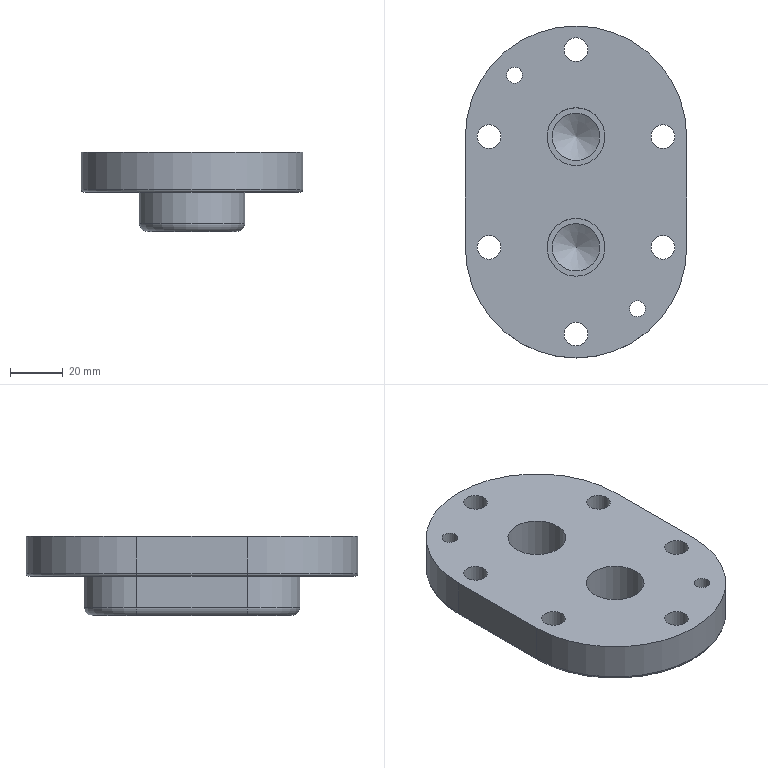Part | NX | features CBORE_HOLE 6, DATUM_CSYS 6, SKETCH 5, SIMPLE HOLE 4, EXTRUDE 3, HOLE PACKAGE 3, BLEND 2 | 1 solid | 45 faces | box 84 x 126 x 30 mm | volume 151500 mm3 | cylinder 24 | plane 15 | torus 4 | cone 2 | commonest cylinder face diameters 9 x6 15 x6 6 x4 2 x2 22 x2 40 x2
STEP:
#1=CARTESIAN_POINT('',(-42.,-21.,15.));
#2=VERTEX_POINT('',#1);
#3=CARTESIAN_POINT('',(-42.,-21.,1.));
#4=VERTEX_POINT('',#3);
#5=CARTESIAN_POINT('',(-42.,-21.,15.));
#6=DIRECTION('',(0.,0.,-1.));
#7=VECTOR('',#6,1000.);
#8=LINE('',#5,#7);
#9=EDGE_CURVE('',#2,#4,#8,.T.);
#10=ORIENTED_EDGE('',*,*,#9,.T.);
#11=CARTESIAN_POINT('',(42.,-21.,1.));
#12=VERTEX_POINT('',#11);
#13=CARTESIAN_POINT('',(0.,-21.,1.));
#14=DIRECTION('',(0.,0.,-1.));
#15=DIRECTION('',(-1.,0.,0.));
#16=AXIS2_PLACEMENT_3D('',#13,#14,#15);
#17=CIRCLE('',#16,42.);
#18=EDGE_CURVE('',#4,#12,#17,.F.);
#19=ORIENTED_EDGE('',*,*,#18,.T.);
#20=CARTESIAN_POINT('',(42.,-21.,15.));
#21=VERTEX_POINT('',#20);
#22=CARTESIAN_POINT('',(42.,-21.,15.));
#23=DIRECTION('',(0.,0.,-1.));
#24=VECTOR('',#23,1000.);
#25=LINE('',#22,#24);
#26=EDGE_CURVE('',#21,#12,#25,.T.);
#27=ORIENTED_EDGE('',*,*,#26,.F.);
#28=CARTESIAN_POINT('',(0.,-21.,15.));
#29=DIRECTION('',(0.,0.,-1.));
#30=DIRECTION('',(1.,0.,0.));
#31=AXIS2_PLACEMENT_3D('',#28,#29,#30);
#32=CIRCLE('',#31,42.);
#33=EDGE_CURVE('',#21,#2,#32,.T.);
#34=ORIENTED_EDGE('',*,*,#33,.T.);
#35=EDGE_LOOP('',(#10,#19,#27,#34));
#36=FACE_BOUND('',#35,.T.);
#37=CARTESIAN_POINT('',(0.,-21.,15.));
#38=DIRECTION('',(0.,0.,-1.));
#39=DIRECTION('',(-1.,0.,0.));
#40=AXIS2_PLACEMENT_3D('',#37,#38,#39);
#41=CYLINDRICAL_SURFACE('',#40,42.);
#42=ADVANCED_FACE('',(#36),#41,.T.);
#43=CARTESIAN_POINT('',(-42.,21.,15.));
#44=VERTEX_POINT('',#43);
#45=CARTESIAN_POINT('',(-42.,21.,1.));
#46=VERTEX_POINT('',#45);
#47=CARTESIAN_POINT('',(-42.,21.,15.));
#48=DIRECTION('',(0.,0.,-1.));
#49=VECTOR('',#48,1000.);
#50=LINE('',#47,#49);
#51=EDGE_CURVE('',#44,#46,#50,.T.);
#52=ORIENTED_EDGE('',*,*,#51,.T.);
#53=CARTESIAN_POINT('',(-42.,-21.,1.));
#54=DIRECTION('',(0.,1.,0.));
#55=VECTOR('',#54,1000.);
#56=LINE('',#53,#55);
#57=EDGE_CURVE('',#46,#4,#56,.F.);
#58=ORIENTED_EDGE('',*,*,#57,.T.);
#59=ORIENTED_EDGE('',*,*,#9,.F.);
#60=CARTESIAN_POINT('',(-42.,-21.,15.));
#61=DIRECTION('',(0.,1.,0.));
#62=VECTOR('',#61,1000.);
#63=LINE('',#60,#62);
#64=EDGE_CURVE('',#2,#44,#63,.T.);
#65=ORIENTED_EDGE('',*,*,#64,.T.);
#66=EDGE_LOOP('',(#52,#58,#59,#65));
#67=FACE_BOUND('',#66,.T.);
#68=CARTESIAN_POINT('',(-42.,-21.,15.));
#69=DIRECTION('',(-1.,0.,0.));
#70=DIRECTION('',(0.,-1.,0.));
#71=AXIS2_PLACEMENT_3D('',#68,#69,#70);
#72=PLANE('',#71);
#73=ADVANCED_FACE('',(#67),#72,.T.);
#74=CARTESIAN_POINT('',(42.,21.,15.));
#75=VERTEX_POINT('',#74);
#76=CARTESIAN_POINT('',(42.,21.,1.));
#77=VERTEX_POINT('',#76);
#78=CARTESIAN_POINT('',(42.,21.,15.));
#79=DIRECTION('',(0.,0.,-1.));
#80=VECTOR('',#79,1000.);
#81=LINE('',#78,#80);
#82=EDGE_CURVE('',#75,#77,#81,.T.);
#83=ORIENTED_EDGE('',*,*,#82,.T.);
#84=CARTESIAN_POINT('',(0.,21.,1.));
#85=DIRECTION('',(0.,0.,-1.));
#86=DIRECTION('',(-1.,0.,0.));
#87=AXIS2_PLACEMENT_3D('',#84,#85,#86);
#88=CIRCLE('',#87,42.);
#89=EDGE_CURVE('',#77,#46,#88,.F.);
#90=ORIENTED_EDGE('',*,*,#89,.T.);
#91=ORIENTED_EDGE('',*,*,#51,.F.);
#92=CARTESIAN_POINT('',(0.,21.,15.));
#93=DIRECTION('',(0.,0.,-1.));
#94=DIRECTION('',(1.,0.,0.));
#95=AXIS2_PLACEMENT_3D('',#92,#93,#94);
#96=CIRCLE('',#95,42.);
#97=EDGE_CURVE('',#44,#75,#96,.T.);
#98=ORIENTED_EDGE('',*,*,#97,.T.);
#99=EDGE_LOOP('',(#83,#90,#91,#98));
#100=FACE_BOUND('',#99,.T.);
#101=CARTESIAN_POINT('',(0.,21.,15.));
#102=DIRECTION('',(0.,0.,-1.));
#103=DIRECTION('',(-1.,0.,0.));
#104=AXIS2_PLACEMENT_3D('',#101,#102,#103);
#105=CYLINDRICAL_SURFACE('',#104,42.);
#106=ADVANCED_FACE('',(#100),#105,.T.);
#107=ORIENTED_EDGE('',*,*,#26,.T.);
#108=CARTESIAN_POINT('',(42.,21.,1.));
#109=DIRECTION('',(0.,-1.,0.));
#110=VECTOR('',#109,1000.);
#111=LINE('',#108,#110);
#112=EDGE_CURVE('',#12,#77,#111,.F.);
#113=ORIENTED_EDGE('',*,*,#112,.T.);
#114=ORIENTED_EDGE('',*,*,#82,.F.);
#115=CARTESIAN_POINT('',(42.,21.,15.));
#116=DIRECTION('',(0.,-1.,0.));
#117=VECTOR('',#116,1000.);
#118=LINE('',#115,#117);
#119=EDGE_CURVE('',#75,#21,#118,.T.);
#120=ORIENTED_EDGE('',*,*,#119,.T.);
#121=EDGE_LOOP('',(#107,#113,#114,#120));
#122=FACE_BOUND('',#121,.T.);
#123=CARTESIAN_POINT('',(42.,21.,15.));
#124=DIRECTION('',(1.,0.,0.));
#125=DIRECTION('',(0.,1.,0.));
#126=AXIS2_PLACEMENT_3D('',#123,#124,#125);
#127=PLANE('',#126);
#128=ADVANCED_FACE('',(#122),#127,.T.);
#129=CARTESIAN_POINT('',(20.335,-44.335,15.));
#130=VERTEX_POINT('',#129);
#131=CARTESIAN_POINT('',(23.335,-44.335,15.));
#132=DIRECTION('',(0.,0.,-1.));
#133=DIRECTION('',(-1.,0.,0.));
#134=AXIS2_PLACEMENT_3D('',#131,#132,#133);
#135=CIRCLE('',#134,3.);
#136=EDGE_CURVE('',#130,#130,#135,.T.);
#137=ORIENTED_EDGE('',*,*,#136,.T.);
#138=EDGE_LOOP('',(#137));
#139=FACE_BOUND('',#138,.T.);
#140=CARTESIAN_POINT('',(-26.335,44.335,15.));
#141=VERTEX_POINT('',#140);
#142=CARTESIAN_POINT('',(-23.335,44.335,15.));
#143=DIRECTION('',(0.,0.,-1.));
#144=DIRECTION('',(-1.,0.,0.));
#145=AXIS2_PLACEMENT_3D('',#142,#143,#144);
#146=CIRCLE('',#145,3.);
#147=EDGE_CURVE('',#141,#141,#146,.T.);
#148=ORIENTED_EDGE('',*,*,#147,.T.);
#149=EDGE_LOOP('',(#148));
#150=FACE_BOUND('',#149,.T.);
#151=CARTESIAN_POINT('',(28.5,21.,15.));
#152=VERTEX_POINT('',#151);
#153=CARTESIAN_POINT('',(33.,21.,15.));
#154=DIRECTION('',(0.,0.,-1.));
#155=DIRECTION('',(-1.,0.,0.));
#156=AXIS2_PLACEMENT_3D('',#153,#154,#155);
#157=CIRCLE('',#156,4.5);
#158=EDGE_CURVE('',#152,#152,#157,.T.);
#159=ORIENTED_EDGE('',*,*,#158,.T.);
#160=EDGE_LOOP('',(#159));
#161=FACE_BOUND('',#160,.T.);
#162=CARTESIAN_POINT('',(28.5,-21.,15.));
#163=VERTEX_POINT('',#162);
#164=CARTESIAN_POINT('',(33.,-21.,15.));
#165=DIRECTION('',(0.,0.,-1.));
#166=DIRECTION('',(-1.,0.,0.));
#167=AXIS2_PLACEMENT_3D('',#164,#165,#166);
#168=CIRCLE('',#167,4.5);
#169=EDGE_CURVE('',#163,#163,#168,.T.);
#170=ORIENTED_EDGE('',*,*,#169,.T.);
#171=EDGE_LOOP('',(#170));
#172=FACE_BOUND('',#171,.T.);
#173=CARTESIAN_POINT('',(-4.5,54.,15.));
#174=VERTEX_POINT('',#173);
#175=CARTESIAN_POINT('',(0.,54.,15.));
#176=DIRECTION('',(0.,0.,-1.));
#177=DIRECTION('',(-1.,0.,0.));
#178=AXIS2_PLACEMENT_3D('',#175,#176,#177);
#179=CIRCLE('',#178,4.5);
#180=EDGE_CURVE('',#174,#174,#179,.T.);
#181=ORIENTED_EDGE('',*,*,#180,.T.);
#182=EDGE_LOOP('',(#181));
#183=FACE_BOUND('',#182,.T.);
#184=CARTESIAN_POINT('',(-4.5,-54.,15.));
#185=VERTEX_POINT('',#184);
#186=CARTESIAN_POINT('',(0.,-54.,15.));
#187=DIRECTION('',(0.,0.,-1.));
#188=DIRECTION('',(-1.,0.,0.));
#189=AXIS2_PLACEMENT_3D('',#186,#187,#188);
#190=CIRCLE('',#189,4.5);
#191=EDGE_CURVE('',#185,#185,#190,.T.);
#192=ORIENTED_EDGE('',*,*,#191,.T.);
#193=EDGE_LOOP('',(#192));
#194=FACE_BOUND('',#193,.T.);
#195=CARTESIAN_POINT('',(-37.5,21.,15.));
#196=VERTEX_POINT('',#195);
#197=CARTESIAN_POINT('',(-33.,21.,15.));
#198=DIRECTION('',(0.,0.,-1.));
#199=DIRECTION('',(-1.,0.,0.));
#200=AXIS2_PLACEMENT_3D('',#197,#198,#199);
#201=CIRCLE('',#200,4.5);
#202=EDGE_CURVE('',#196,#196,#201,.T.);
#203=ORIENTED_EDGE('',*,*,#202,.T.);
#204=EDGE_LOOP('',(#203));
#205=FACE_BOUND('',#204,.T.);
#206=CARTESIAN_POINT('',(-37.5,-21.,15.));
#207=VERTEX_POINT('',#206);
#208=CARTESIAN_POINT('',(-33.,-21.,15.));
#209=DIRECTION('',(0.,0.,-1.));
#210=DIRECTION('',(-1.,0.,0.));
#211=AXIS2_PLACEMENT_3D('',#208,#209,#210);
#212=CIRCLE('',#211,4.5);
#213=EDGE_CURVE('',#207,#207,#212,.T.);
#214=ORIENTED_EDGE('',*,*,#213,.T.);
#215=EDGE_LOOP('',(#214));
#216=FACE_BOUND('',#215,.T.);
#217=CARTESIAN_POINT('',(0.,32.,15.));
#218=VERTEX_POINT('',#217);
#219=CARTESIAN_POINT('',(0.,21.,15.));
#220=DIRECTION('',(0.,0.,1.));
#221=DIRECTION('',(0.,1.,0.));
#222=AXIS2_PLACEMENT_3D('',#219,#220,#221);
#223=CIRCLE('',#222,11.);
#224=EDGE_CURVE('',#218,#218,#223,.T.);
#225=ORIENTED_EDGE('',*,*,#224,.F.);
#226=EDGE_LOOP('',(#225));
#227=FACE_BOUND('',#226,.T.);
#228=CARTESIAN_POINT('',(0.,-10.,15.));
#229=VERTEX_POINT('',#228);
#230=CARTESIAN_POINT('',(0.,-21.,15.));
#231=DIRECTION('',(0.,0.,1.));
#232=DIRECTION('',(0.,1.,0.));
#233=AXIS2_PLACEMENT_3D('',#230,#231,#232);
#234=CIRCLE('',#233,11.);
#235=EDGE_CURVE('',#229,#229,#234,.T.);
#236=ORIENTED_EDGE('',*,*,#235,.F.);
#237=EDGE_LOOP('',(#236));
#238=FACE_BOUND('',#237,.T.);
#239=ORIENTED_EDGE('',*,*,#33,.F.);
#240=ORIENTED_EDGE('',*,*,#119,.F.);
#241=ORIENTED_EDGE('',*,*,#97,.F.);
#242=ORIENTED_EDGE('',*,*,#64,.F.);
#243=EDGE_LOOP('',(#239,#240,#241,#242));
#244=FACE_BOUND('',#243,.T.);
#245=CARTESIAN_POINT('',(0.,-21.,15.));
#246=DIRECTION('',(0.,0.,-1.));
#247=DIRECTION('',(-1.,0.,0.));
#248=AXIS2_PLACEMENT_3D('',#245,#246,#247);
#249=PLANE('',#248);
#250=ADVANCED_FACE('',(#139,#150,#161,#172,#183,#194,#205,#216,#227,#238,#244),#249,.F.);
#251=CARTESIAN_POINT('',(26.335,-44.335,0.));
#252=VERTEX_POINT('',#251);
#253=CARTESIAN_POINT('',(23.335,-44.335,0.));
#254=DIRECTION('',(0.,0.,1.));
#255=DIRECTION('',(1.,0.,0.));
#256=AXIS2_PLACEMENT_3D('',#253,#254,#255);
#257=CIRCLE('',#256,3.);
#258=EDGE_CURVE('',#252,#252,#257,.T.);
#259=ORIENTED_EDGE('',*,*,#258,.T.);
#260=EDGE_LOOP('',(#259));
#261=FACE_BOUND('',#260,.T.);
#262=CARTESIAN_POINT('',(-20.335,44.335,0.));
#263=VERTEX_POINT('',#262);
#264=CARTESIAN_POINT('',(-23.335,44.335,0.));
#265=DIRECTION('',(0.,0.,1.));
#266=DIRECTION('',(1.,0.,0.));
#267=AXIS2_PLACEMENT_3D('',#264,#265,#266);
#268=CIRCLE('',#267,3.);
#269=EDGE_CURVE('',#263,#263,#268,.T.);
#270=ORIENTED_EDGE('',*,*,#269,.T.);
#271=EDGE_LOOP('',(#270));
#272=FACE_BOUND('',#271,.T.);
#273=CARTESIAN_POINT('',(-41.,21.,0.));
#274=VERTEX_POINT('',#273);
#275=CARTESIAN_POINT('',(41.,21.,0.));
#276=VERTEX_POINT('',#275);
#277=CARTESIAN_POINT('',(0.,21.,0.));
#278=DIRECTION('',(0.,0.,-1.));
#279=DIRECTION('',(-1.,0.,0.));
#280=AXIS2_PLACEMENT_3D('',#277,#278,#279);
#281=CIRCLE('',#280,41.);
#282=EDGE_CURVE('',#274,#276,#281,.T.);
#283=ORIENTED_EDGE('',*,*,#282,.T.);
#284=CARTESIAN_POINT('',(41.,-21.,0.));
#285=VERTEX_POINT('',#284);
#286=CARTESIAN_POINT('',(41.,-21.,0.));
#287=DIRECTION('',(0.,-1.,0.));
#288=VECTOR('',#287,1000.);
#289=LINE('',#286,#288);
#290=EDGE_CURVE('',#276,#285,#289,.T.);
#291=ORIENTED_EDGE('',*,*,#290,.T.);
#292=CARTESIAN_POINT('',(-41.,-21.,0.));
#293=VERTEX_POINT('',#292);
#294=CARTESIAN_POINT('',(0.,-21.,0.));
#295=DIRECTION('',(0.,0.,-1.));
#296=DIRECTION('',(-1.,0.,0.));
#297=AXIS2_PLACEMENT_3D('',#294,#295,#296);
#298=CIRCLE('',#297,41.);
#299=EDGE_CURVE('',#285,#293,#298,.T.);
#300=ORIENTED_EDGE('',*,*,#299,.T.);
#301=CARTESIAN_POINT('',(-41.,-21.,0.));
#302=DIRECTION('',(0.,1.,0.));
#303=VECTOR('',#302,1000.);
#304=LINE('',#301,#303);
#305=EDGE_CURVE('',#293,#274,#304,.T.);
#306=ORIENTED_EDGE('',*,*,#305,.T.);
#307=EDGE_LOOP('',(#283,#291,#300,#306));
#308=FACE_BOUND('',#307,.T.);
#309=CARTESIAN_POINT('',(40.5,21.,0.));
#310=VERTEX_POINT('',#309);
#311=CARTESIAN_POINT('',(33.,21.,0.));
#312=DIRECTION('',(0.,0.,1.));
#313=DIRECTION('',(1.,0.,0.));
#314=AXIS2_PLACEMENT_3D('',#311,#312,#313);
#315=CIRCLE('',#314,7.5);
#316=EDGE_CURVE('',#310,#310,#315,.T.);
#317=ORIENTED_EDGE('',*,*,#316,.T.);
#318=EDGE_LOOP('',(#317));
#319=FACE_BOUND('',#318,.T.);
#320=CARTESIAN_POINT('',(40.5,-21.,0.));
#321=VERTEX_POINT('',#320);
#322=CARTESIAN_POINT('',(33.,-21.,0.));
#323=DIRECTION('',(0.,0.,1.));
#324=DIRECTION('',(1.,0.,0.));
#325=AXIS2_PLACEMENT_3D('',#322,#323,#324);
#326=CIRCLE('',#325,7.5);
#327=EDGE_CURVE('',#321,#321,#326,.T.);
#328=ORIENTED_EDGE('',*,*,#327,.T.);
#329=EDGE_LOOP('',(#328));
#330=FACE_BOUND('',#329,.T.);
#331=CARTESIAN_POINT('',(7.5,54.,0.));
#332=VERTEX_POINT('',#331);
#333=CARTESIAN_POINT('',(0.,54.,0.));
#334=DIRECTION('',(0.,0.,1.));
#335=DIRECTION('',(1.,0.,0.));
#336=AXIS2_PLACEMENT_3D('',#333,#334,#335);
#337=CIRCLE('',#336,7.5);
#338=EDGE_CURVE('',#332,#332,#337,.T.);
#339=ORIENTED_EDGE('',*,*,#338,.T.);
#340=EDGE_LOOP('',(#339));
#341=FACE_BOUND('',#340,.T.);
#342=CARTESIAN_POINT('',(7.5,-54.,0.));
#343=VERTEX_POINT('',#342);
#344=CARTESIAN_POINT('',(0.,-54.,0.));
#345=DIRECTION('',(0.,0.,1.));
#346=DIRECTION('',(1.,0.,0.));
#347=AXIS2_PLACEMENT_3D('',#344,#345,#346);
#348=CIRCLE('',#347,7.5);
#349=EDGE_CURVE('',#343,#343,#348,.T.);
#350=ORIENTED_EDGE('',*,*,#349,.T.);
#351=EDGE_LOOP('',(#350));
#352=FACE_BOUND('',#351,.T.);
#353=CARTESIAN_POINT('',(-25.5,21.,0.));
#354=VERTEX_POINT('',#353);
#355=CARTESIAN_POINT('',(-33.,21.,0.));
#356=DIRECTION('',(0.,0.,1.));
#357=DIRECTION('',(1.,0.,0.));
#358=AXIS2_PLACEMENT_3D('',#355,#356,#357);
#359=CIRCLE('',#358,7.5);
#360=EDGE_CURVE('',#354,#354,#359,.T.);
#361=ORIENTED_EDGE('',*,*,#360,.T.);
#362=EDGE_LOOP('',(#361));
#363=FACE_BOUND('',#362,.T.);
#364=CARTESIAN_POINT('',(-25.5,-21.,0.));
#365=VERTEX_POINT('',#364);
#366=CARTESIAN_POINT('',(-33.,-21.,0.));
#367=DIRECTION('',(0.,0.,1.));
#368=DIRECTION('',(1.,0.,0.));
#369=AXIS2_PLACEMENT_3D('',#366,#367,#368);
#370=CIRCLE('',#369,7.5);
#371=EDGE_CURVE('',#365,#365,#370,.T.);
#372=ORIENTED_EDGE('',*,*,#371,.T.);
#373=EDGE_LOOP('',(#372));
#374=FACE_BOUND('',#373,.T.);
#375=CARTESIAN_POINT('',(-20.,-21.,0.));
#376=VERTEX_POINT('',#375);
#377=CARTESIAN_POINT('',(-20.,21.,0.));
#378=VERTEX_POINT('',#377);
#379=CARTESIAN_POINT('',(-20.,-21.,0.));
#380=DIRECTION('',(0.,1.,0.));
#381=VECTOR('',#380,1000.);
#382=LINE('',#379,#381);
#383=EDGE_CURVE('',#376,#378,#382,.T.);
#384=ORIENTED_EDGE('',*,*,#383,.F.);
#385=CARTESIAN_POINT('',(20.,-21.,0.));
#386=VERTEX_POINT('',#385);
#387=CARTESIAN_POINT('',(0.,-21.,0.));
#388=DIRECTION('',(0.,0.,-1.));
#389=DIRECTION('',(1.,0.,0.));
#390=AXIS2_PLACEMENT_3D('',#387,#388,#389);
#391=CIRCLE('',#390,20.);
#392=EDGE_CURVE('',#386,#376,#391,.T.);
#393=ORIENTED_EDGE('',*,*,#392,.F.);
#394=CARTESIAN_POINT('',(20.,21.,0.));
#395=VERTEX_POINT('',#394);
#396=CARTESIAN_POINT('',(20.,21.,0.));
#397=DIRECTION('',(0.,-1.,0.));
#398=VECTOR('',#397,1000.);
#399=LINE('',#396,#398);
#400=EDGE_CURVE('',#395,#386,#399,.T.);
#401=ORIENTED_EDGE('',*,*,#400,.F.);
#402=CARTESIAN_POINT('',(0.,21.,0.));
#403=DIRECTION('',(0.,0.,-1.));
#404=DIRECTION('',(1.,0.,0.));
#405=AXIS2_PLACEMENT_3D('',#402,#403,#404);
#406=CIRCLE('',#405,20.);
#407=EDGE_CURVE('',#378,#395,#406,.T.);
#408=ORIENTED_EDGE('',*,*,#407,.F.);
#409=EDGE_LOOP('',(#384,#393,#401,#408));
#410=FACE_BOUND('',#409,.T.);
#411=CARTESIAN_POINT('',(0.,-21.,0.));
#412=DIRECTION('',(0.,0.,-1.));
#413=DIRECTION('',(-1.,0.,0.));
#414=AXIS2_PLACEMENT_3D('',#411,#412,#413);
#415=PLANE('',#414);
#416=ADVANCED_FACE('',(#261,#272,#308,#319,#330,#341,#352,#363,#374,#410),#415,.T.);
#417=CARTESIAN_POINT('',(-20.,21.,-12.));
#418=VERTEX_POINT('',#417);
#419=CARTESIAN_POINT('',(-20.,21.,-15.));
#420=DIRECTION('',(0.,0.,1.));
#421=VECTOR('',#420,1000.);
#422=LINE('',#419,#421);
#423=EDGE_CURVE('',#418,#378,#422,.T.);
#424=ORIENTED_EDGE('',*,*,#423,.F.);
#425=CARTESIAN_POINT('',(-20.,-21.,-12.));
#426=VERTEX_POINT('',#425);
#427=CARTESIAN_POINT('',(-20.,-21.,-12.));
#428=DIRECTION('',(0.,1.,0.));
#429=VECTOR('',#428,1000.);
#430=LINE('',#427,#429);
#431=EDGE_CURVE('',#418,#426,#430,.F.);
#432=ORIENTED_EDGE('',*,*,#431,.T.);
#433=CARTESIAN_POINT('',(-20.,-21.,-15.));
#434=DIRECTION('',(0.,0.,1.));
#435=VECTOR('',#434,1000.);
#436=LINE('',#433,#435);
#437=EDGE_CURVE('',#426,#376,#436,.T.);
#438=ORIENTED_EDGE('',*,*,#437,.T.);
#439=ORIENTED_EDGE('',*,*,#383,.T.);
#440=EDGE_LOOP('',(#424,#432,#438,#439));
#441=FACE_BOUND('',#440,.T.);
#442=CARTESIAN_POINT('',(-20.,-21.,-15.));
#443=DIRECTION('',(1.,0.,0.));
#444=DIRECTION('',(0.,1.,0.));
#445=AXIS2_PLACEMENT_3D('',#442,#443,#444);
#446=PLANE('',#445);
#447=ADVANCED_FACE('',(#441),#446,.F.);
#448=CARTESIAN_POINT('',(20.,21.,-12.));
#449=VERTEX_POINT('',#448);
#450=CARTESIAN_POINT('',(20.,21.,-15.));
#451=DIRECTION('',(0.,0.,1.));
#452=VECTOR('',#451,1000.);
#453=LINE('',#450,#452);
#454=EDGE_CURVE('',#449,#395,#453,.T.);
#455=ORIENTED_EDGE('',*,*,#454,.F.);
#456=CARTESIAN_POINT('',(0.,21.,-12.));
#457=DIRECTION('',(0.,0.,-1.));
#458=DIRECTION('',(-1.,0.,0.));
#459=AXIS2_PLACEMENT_3D('',#456,#457,#458);
#460=CIRCLE('',#459,20.);
#461=EDGE_CURVE('',#449,#418,#460,.F.);
#462=ORIENTED_EDGE('',*,*,#461,.T.);
#463=ORIENTED_EDGE('',*,*,#423,.T.);
#464=ORIENTED_EDGE('',*,*,#407,.T.);
#465=EDGE_LOOP('',(#455,#462,#463,#464));
#466=FACE_BOUND('',#465,.T.);
#467=CARTESIAN_POINT('',(0.,21.,-15.));
#468=DIRECTION('',(0.,0.,1.));
#469=DIRECTION('',(1.,0.,0.));
#470=AXIS2_PLACEMENT_3D('',#467,#468,#469);
#471=CYLINDRICAL_SURFACE('',#470,20.);
#472=ADVANCED_FACE('',(#466),#471,.T.);
#473=CARTESIAN_POINT('',(20.,-21.,-12.));
#474=VERTEX_POINT('',#473);
#475=CARTESIAN_POINT('',(20.,-21.,-15.));
#476=DIRECTION('',(0.,0.,1.));
#477=VECTOR('',#476,1000.);
#478=LINE('',#475,#477);
#479=EDGE_CURVE('',#474,#386,#478,.T.);
#480=ORIENTED_EDGE('',*,*,#479,.F.);
#481=CARTESIAN_POINT('',(20.,21.,-12.));
#482=DIRECTION('',(0.,-1.,0.));
#483=VECTOR('',#482,1000.);
#484=LINE('',#481,#483);
#485=EDGE_CURVE('',#474,#449,#484,.F.);
#486=ORIENTED_EDGE('',*,*,#485,.T.);
#487=ORIENTED_EDGE('',*,*,#454,.T.);
#488=ORIENTED_EDGE('',*,*,#400,.T.);
#489=EDGE_LOOP('',(#480,#486,#487,#488));
#490=FACE_BOUND('',#489,.T.);
#491=CARTESIAN_POINT('',(20.,21.,-15.));
#492=DIRECTION('',(-1.,0.,0.));
#493=DIRECTION('',(0.,-1.,0.));
#494=AXIS2_PLACEMENT_3D('',#491,#492,#493);
#495=PLANE('',#494);
#496=ADVANCED_FACE('',(#490),#495,.F.);
#497=ORIENTED_EDGE('',*,*,#437,.F.);
#498=CARTESIAN_POINT('',(0.,-21.,-12.));
#499=DIRECTION('',(0.,0.,-1.));
#500=DIRECTION('',(-1.,0.,0.));
#501=AXIS2_PLACEMENT_3D('',#498,#499,#500);
#502=CIRCLE('',#501,20.);
#503=EDGE_CURVE('',#426,#474,#502,.F.);
#504=ORIENTED_EDGE('',*,*,#503,.T.);
#505=ORIENTED_EDGE('',*,*,#479,.T.);
#506=ORIENTED_EDGE('',*,*,#392,.T.);
#507=EDGE_LOOP('',(#497,#504,#505,#506));
#508=FACE_BOUND('',#507,.T.);
#509=CARTESIAN_POINT('',(0.,-21.,-15.));
#510=DIRECTION('',(0.,0.,1.));
#511=DIRECTION('',(1.,0.,0.));
#512=AXIS2_PLACEMENT_3D('',#509,#510,#511);
#513=CYLINDRICAL_SURFACE('',#512,20.);
#514=ADVANCED_FACE('',(#508),#513,.T.);
#515=CARTESIAN_POINT('',(-17.,21.,-15.));
#516=VERTEX_POINT('',#515);
#517=CARTESIAN_POINT('',(17.,21.,-15.));
#518=VERTEX_POINT('',#517);
#519=CARTESIAN_POINT('',(0.,21.,-15.));
#520=DIRECTION('',(0.,0.,-1.));
#521=DIRECTION('',(-1.,0.,0.));
#522=AXIS2_PLACEMENT_3D('',#519,#520,#521);
#523=CIRCLE('',#522,17.);
#524=EDGE_CURVE('',#516,#518,#523,.T.);
#525=ORIENTED_EDGE('',*,*,#524,.T.);
#526=CARTESIAN_POINT('',(17.,-21.,-15.));
#527=VERTEX_POINT('',#526);
#528=CARTESIAN_POINT('',(17.,-21.,-15.));
#529=DIRECTION('',(0.,-1.,0.));
#530=VECTOR('',#529,1000.);
#531=LINE('',#528,#530);
#532=EDGE_CURVE('',#518,#527,#531,.T.);
#533=ORIENTED_EDGE('',*,*,#532,.T.);
#534=CARTESIAN_POINT('',(-17.,-21.,-15.));
#535=VERTEX_POINT('',#534);
#536=CARTESIAN_POINT('',(0.,-21.,-15.));
#537=DIRECTION('',(0.,0.,-1.));
#538=DIRECTION('',(-1.,0.,0.));
#539=AXIS2_PLACEMENT_3D('',#536,#537,#538);
#540=CIRCLE('',#539,17.);
#541=EDGE_CURVE('',#527,#535,#540,.T.);
#542=ORIENTED_EDGE('',*,*,#541,.T.);
#543=CARTESIAN_POINT('',(-17.,21.,-15.));
#544=DIRECTION('',(0.,1.,0.));
#545=VECTOR('',#544,1000.);
#546=LINE('',#543,#545);
#547=EDGE_CURVE('',#535,#516,#546,.T.);
#548=ORIENTED_EDGE('',*,*,#547,.T.);
#549=EDGE_LOOP('',(#525,#533,#542,#548));
#550=FACE_BOUND('',#549,.T.);
#551=CARTESIAN_POINT('',(0.,21.,-15.));
#552=DIRECTION('',(0.,0.,-1.));
#553=DIRECTION('',(-1.,0.,0.));
#554=AXIS2_PLACEMENT_3D('',#551,#552,#553);
#555=PLANE('',#554);
#556=ADVANCED_FACE('',(#550),#555,.T.);
#557=CARTESIAN_POINT('',(0.,32.,-5.));
#558=VERTEX_POINT('',#557);
#559=CARTESIAN_POINT('',(0.,21.,-5.));
#560=DIRECTION('',(0.,0.,1.));
#561=DIRECTION('',(0.,1.,0.));
#562=AXIS2_PLACEMENT_3D('',#559,#560,#561);
#563=CIRCLE('',#562,11.);
#564=EDGE_CURVE('',#558,#558,#563,.F.);
#565=ORIENTED_EDGE('',*,*,#564,.F.);
#566=EDGE_LOOP('',(#565));
#567=FACE_BOUND('',#566,.T.);
#568=CARTESIAN_POINT('',(9.,21.,-5.));
#569=VERTEX_POINT('',#568);
#570=CARTESIAN_POINT('',(0.,21.,-5.));
#571=DIRECTION('',(0.,0.,1.));
#572=DIRECTION('',(1.,0.,0.));
#573=AXIS2_PLACEMENT_3D('',#570,#571,#572);
#574=CIRCLE('',#573,9.);
#575=EDGE_CURVE('',#569,#569,#574,.F.);
#576=ORIENTED_EDGE('',*,*,#575,.T.);
#577=EDGE_LOOP('',(#576));
#578=FACE_BOUND('',#577,.T.);
#579=CARTESIAN_POINT('',(0.,21.,-5.));
#580=DIRECTION('',(0.,0.,1.));
#581=DIRECTION('',(1.,0.,0.));
#582=AXIS2_PLACEMENT_3D('',#579,#580,#581);
#583=PLANE('',#582);
#584=ADVANCED_FACE('',(#567,#578),#583,.T.);
#585=ORIENTED_EDGE('',*,*,#564,.T.);
#586=EDGE_LOOP('',(#585));
#587=FACE_BOUND('',#586,.T.);
#588=ORIENTED_EDGE('',*,*,#224,.T.);
#589=EDGE_LOOP('',(#588));
#590=FACE_BOUND('',#589,.T.);
#591=CARTESIAN_POINT('',(0.,21.,-5.));
#592=DIRECTION('',(0.,0.,1.));
#593=DIRECTION('',(1.,0.,0.));
#594=AXIS2_PLACEMENT_3D('',#591,#592,#593);
#595=CYLINDRICAL_SURFACE('',#594,11.);
#596=ADVANCED_FACE('',(#587,#590),#595,.F.);
#597=CARTESIAN_POINT('',(0.,-10.,-5.));
#598=VERTEX_POINT('',#597);
#599=CARTESIAN_POINT('',(0.,-21.,-5.));
#600=DIRECTION('',(0.,0.,1.));
#601=DIRECTION('',(0.,1.,0.));
#602=AXIS2_PLACEMENT_3D('',#599,#600,#601);
#603=CIRCLE('',#602,11.);
#604=EDGE_CURVE('',#598,#598,#603,.F.);
#605=ORIENTED_EDGE('',*,*,#604,.F.);
#606=EDGE_LOOP('',(#605));
#607=FACE_BOUND('',#606,.T.);
#608=CARTESIAN_POINT('',(9.,-21.,-5.));
#609=VERTEX_POINT('',#608);
#610=CARTESIAN_POINT('',(0.,-21.,-5.));
#611=DIRECTION('',(0.,0.,1.));
#612=DIRECTION('',(1.,0.,0.));
#613=AXIS2_PLACEMENT_3D('',#610,#611,#612);
#614=CIRCLE('',#613,9.);
#615=EDGE_CURVE('',#609,#609,#614,.F.);
#616=ORIENTED_EDGE('',*,*,#615,.T.);
#617=EDGE_LOOP('',(#616));
#618=FACE_BOUND('',#617,.T.);
#619=CARTESIAN_POINT('',(0.,-21.,-5.));
#620=DIRECTION('',(0.,0.,1.));
#621=DIRECTION('',(1.,0.,0.));
#622=AXIS2_PLACEMENT_3D('',#619,#620,#621);
#623=PLANE('',#622);
#624=ADVANCED_FACE('',(#607,#618),#623,.T.);
#625=ORIENTED_EDGE('',*,*,#604,.T.);
#626=EDGE_LOOP('',(#625));
#627=FACE_BOUND('',#626,.T.);
#628=ORIENTED_EDGE('',*,*,#235,.T.);
#629=EDGE_LOOP('',(#628));
#630=FACE_BOUND('',#629,.T.);
#631=CARTESIAN_POINT('',(0.,-21.,-5.));
#632=DIRECTION('',(0.,0.,1.));
#633=DIRECTION('',(1.,0.,0.));
#634=AXIS2_PLACEMENT_3D('',#631,#632,#633);
#635=CYLINDRICAL_SURFACE('',#634,11.);
#636=ADVANCED_FACE('',(#627,#630),#635,.F.);
#637=ORIENTED_EDGE('',*,*,#575,.F.);
#638=EDGE_LOOP('',(#637));
#639=FACE_BOUND('',#638,.T.);
#640=CARTESIAN_POINT('',(0.,21.,-10.408));
#641=VERTEX_POINT('',#640);
#642=VERTEX_LOOP('',#641);
#643=FACE_BOUND('',#642,.T.);
#644=CARTESIAN_POINT('',(0.,21.,-5.));
#645=DIRECTION('',(0.,0.,1.));
#646=DIRECTION('',(1.,0.,0.));
#647=AXIS2_PLACEMENT_3D('',#644,#645,#646);
#648=CONICAL_SURFACE('',#647,9.,1.03);
#649=ADVANCED_FACE('',(#639,#643),#648,.F.);
#650=ORIENTED_EDGE('',*,*,#615,.F.);
#651=EDGE_LOOP('',(#650));
#652=FACE_BOUND('',#651,.T.);
#653=CARTESIAN_POINT('',(0.,-21.,-10.408));
#654=VERTEX_POINT('',#653);
#655=VERTEX_LOOP('',#654);
#656=FACE_BOUND('',#655,.T.);
#657=CARTESIAN_POINT('',(0.,-21.,-5.));
#658=DIRECTION('',(0.,0.,1.));
#659=DIRECTION('',(1.,0.,0.));
#660=AXIS2_PLACEMENT_3D('',#657,#658,#659);
#661=CONICAL_SURFACE('',#660,9.,1.03);
#662=ADVANCED_FACE('',(#652,#656),#661,.F.);
#663=CARTESIAN_POINT('',(-28.5,-21.,8.));
#664=VERTEX_POINT('',#663);
#665=CARTESIAN_POINT('',(-33.,-21.,8.));
#666=DIRECTION('',(0.,0.,1.));
#667=DIRECTION('',(1.,0.,0.));
#668=AXIS2_PLACEMENT_3D('',#665,#666,#667);
#669=CIRCLE('',#668,4.5);
#670=EDGE_CURVE('',#664,#664,#669,.F.);
#671=ORIENTED_EDGE('',*,*,#670,.T.);
#672=EDGE_LOOP('',(#671));
#673=FACE_BOUND('',#672,.T.);
#674=ORIENTED_EDGE('',*,*,#213,.F.);
#675=EDGE_LOOP('',(#674));
#676=FACE_BOUND('',#675,.T.);
#677=CARTESIAN_POINT('',(-33.,-21.,20.));
#678=DIRECTION('',(0.,0.,1.));
#679=DIRECTION('',(1.,0.,0.));
#680=AXIS2_PLACEMENT_3D('',#677,#678,#679);
#681=CYLINDRICAL_SURFACE('',#680,4.5);
#682=ADVANCED_FACE('',(#673,#676),#681,.F.);
#683=ORIENTED_EDGE('',*,*,#670,.F.);
#684=EDGE_LOOP('',(#683));
#685=FACE_BOUND('',#684,.T.);
#686=CARTESIAN_POINT('',(-25.5,-21.,8.));
#687=VERTEX_POINT('',#686);
#688=CARTESIAN_POINT('',(-33.,-21.,8.));
#689=DIRECTION('',(0.,0.,1.));
#690=DIRECTION('',(1.,0.,0.));
#691=AXIS2_PLACEMENT_3D('',#688,#689,#690);
#692=CIRCLE('',#691,7.5);
#693=EDGE_CURVE('',#687,#687,#692,.F.);
#694=ORIENTED_EDGE('',*,*,#693,.T.);
#695=EDGE_LOOP('',(#694));
#696=FACE_BOUND('',#695,.T.);
#697=CARTESIAN_POINT('',(-33.,-21.,8.));
#698=DIRECTION('',(0.,0.,1.));
#699=DIRECTION('',(1.,0.,0.));
#700=AXIS2_PLACEMENT_3D('',#697,#698,#699);
#701=PLANE('',#700);
#702=ADVANCED_FACE('',(#685,#696),#701,.F.);
#703=ORIENTED_EDGE('',*,*,#693,.F.);
#704=EDGE_LOOP('',(#703));
#705=FACE_BOUND('',#704,.T.);
#706=ORIENTED_EDGE('',*,*,#371,.F.);
#707=EDGE_LOOP('',(#706));
#708=FACE_BOUND('',#707,.T.);
#709=CARTESIAN_POINT('',(-33.,-21.,0.));
#710=DIRECTION('',(0.,0.,1.));
#711=DIRECTION('',(1.,0.,0.));
#712=AXIS2_PLACEMENT_3D('',#709,#710,#711);
#713=CYLINDRICAL_SURFACE('',#712,7.5);
#714=ADVANCED_FACE('',(#705,#708),#713,.F.);
#715=CARTESIAN_POINT('',(-28.5,21.,8.));
#716=VERTEX_POINT('',#715);
#717=CARTESIAN_POINT('',(-33.,21.,8.));
#718=DIRECTION('',(0.,0.,1.));
#719=DIRECTION('',(1.,0.,0.));
#720=AXIS2_PLACEMENT_3D('',#717,#718,#719);
#721=CIRCLE('',#720,4.5);
#722=EDGE_CURVE('',#716,#716,#721,.F.);
#723=ORIENTED_EDGE('',*,*,#722,.T.);
#724=EDGE_LOOP('',(#723));
#725=FACE_BOUND('',#724,.T.);
#726=ORIENTED_EDGE('',*,*,#202,.F.);
#727=EDGE_LOOP('',(#726));
#728=FACE_BOUND('',#727,.T.);
#729=CARTESIAN_POINT('',(-33.,21.,20.));
#730=DIRECTION('',(0.,0.,1.));
#731=DIRECTION('',(1.,0.,0.));
#732=AXIS2_PLACEMENT_3D('',#729,#730,#731);
#733=CYLINDRICAL_SURFACE('',#732,4.5);
#734=ADVANCED_FACE('',(#725,#728),#733,.F.);
#735=ORIENTED_EDGE('',*,*,#722,.F.);
#736=EDGE_LOOP('',(#735));
#737=FACE_BOUND('',#736,.T.);
#738=CARTESIAN_POINT('',(-25.5,21.,8.));
#739=VERTEX_POINT('',#738);
#740=CARTESIAN_POINT('',(-33.,21.,8.));
#741=DIRECTION('',(0.,0.,1.));
#742=DIRECTION('',(1.,0.,0.));
#743=AXIS2_PLACEMENT_3D('',#740,#741,#742);
#744=CIRCLE('',#743,7.5);
#745=EDGE_CURVE('',#739,#739,#744,.F.);
#746=ORIENTED_EDGE('',*,*,#745,.T.);
#747=EDGE_LOOP('',(#746));
#748=FACE_BOUND('',#747,.T.);
#749=CARTESIAN_POINT('',(-33.,21.,8.));
#750=DIRECTION('',(0.,0.,1.));
#751=DIRECTION('',(1.,0.,0.));
#752=AXIS2_PLACEMENT_3D('',#749,#750,#751);
#753=PLANE('',#752);
#754=ADVANCED_FACE('',(#737,#748),#753,.F.);
#755=ORIENTED_EDGE('',*,*,#745,.F.);
#756=EDGE_LOOP('',(#755));
#757=FACE_BOUND('',#756,.T.);
#758=ORIENTED_EDGE('',*,*,#360,.F.);
#759=EDGE_LOOP('',(#758));
#760=FACE_BOUND('',#759,.T.);
#761=CARTESIAN_POINT('',(-33.,21.,0.));
#762=DIRECTION('',(0.,0.,1.));
#763=DIRECTION('',(1.,0.,0.));
#764=AXIS2_PLACEMENT_3D('',#761,#762,#763);
#765=CYLINDRICAL_SURFACE('',#764,7.5);
#766=ADVANCED_FACE('',(#757,#760),#765,.F.);
#767=CARTESIAN_POINT('',(4.5,-54.,8.));
#768=VERTEX_POINT('',#767);
#769=CARTESIAN_POINT('',(0.,-54.,8.));
#770=DIRECTION('',(0.,0.,1.));
#771=DIRECTION('',(1.,0.,0.));
#772=AXIS2_PLACEMENT_3D('',#769,#770,#771);
#773=CIRCLE('',#772,4.5);
#774=EDGE_CURVE('',#768,#768,#773,.F.);
#775=ORIENTED_EDGE('',*,*,#774,.T.);
#776=EDGE_LOOP('',(#775));
#777=FACE_BOUND('',#776,.T.);
#778=ORIENTED_EDGE('',*,*,#191,.F.);
#779=EDGE_LOOP('',(#778));
#780=FACE_BOUND('',#779,.T.);
#781=CARTESIAN_POINT('',(0.,-54.,20.));
#782=DIRECTION('',(0.,0.,1.));
#783=DIRECTION('',(1.,0.,0.));
#784=AXIS2_PLACEMENT_3D('',#781,#782,#783);
#785=CYLINDRICAL_SURFACE('',#784,4.5);
#786=ADVANCED_FACE('',(#777,#780),#785,.F.);
#787=ORIENTED_EDGE('',*,*,#774,.F.);
#788=EDGE_LOOP('',(#787));
#789=FACE_BOUND('',#788,.T.);
#790=CARTESIAN_POINT('',(7.5,-54.,8.));
#791=VERTEX_POINT('',#790);
#792=CARTESIAN_POINT('',(0.,-54.,8.));
#793=DIRECTION('',(0.,0.,1.));
#794=DIRECTION('',(1.,0.,0.));
#795=AXIS2_PLACEMENT_3D('',#792,#793,#794);
#796=CIRCLE('',#795,7.5);
#797=EDGE_CURVE('',#791,#791,#796,.F.);
#798=ORIENTED_EDGE('',*,*,#797,.T.);
#799=EDGE_LOOP('',(#798));
#800=FACE_BOUND('',#799,.T.);
#801=CARTESIAN_POINT('',(0.,-54.,8.));
#802=DIRECTION('',(0.,0.,1.));
#803=DIRECTION('',(1.,0.,0.));
#804=AXIS2_PLACEMENT_3D('',#801,#802,#803);
#805=PLANE('',#804);
#806=ADVANCED_FACE('',(#789,#800),#805,.F.);
#807=ORIENTED_EDGE('',*,*,#797,.F.);
#808=EDGE_LOOP('',(#807));
#809=FACE_BOUND('',#808,.T.);
#810=ORIENTED_EDGE('',*,*,#349,.F.);
#811=EDGE_LOOP('',(#810));
#812=FACE_BOUND('',#811,.T.);
#813=CARTESIAN_POINT('',(0.,-54.,0.));
#814=DIRECTION('',(0.,0.,1.));
#815=DIRECTION('',(1.,0.,0.));
#816=AXIS2_PLACEMENT_3D('',#813,#814,#815);
#817=CYLINDRICAL_SURFACE('',#816,7.5);
#818=ADVANCED_FACE('',(#809,#812),#817,.F.);
#819=CARTESIAN_POINT('',(4.5,54.,8.));
#820=VERTEX_POINT('',#819);
#821=CARTESIAN_POINT('',(0.,54.,8.));
#822=DIRECTION('',(0.,0.,1.));
#823=DIRECTION('',(1.,0.,0.));
#824=AXIS2_PLACEMENT_3D('',#821,#822,#823);
#825=CIRCLE('',#824,4.5);
#826=EDGE_CURVE('',#820,#820,#825,.F.);
#827=ORIENTED_EDGE('',*,*,#826,.T.);
#828=EDGE_LOOP('',(#827));
#829=FACE_BOUND('',#828,.T.);
#830=ORIENTED_EDGE('',*,*,#180,.F.);
#831=EDGE_LOOP('',(#830));
#832=FACE_BOUND('',#831,.T.);
#833=CARTESIAN_POINT('',(0.,54.,20.));
#834=DIRECTION('',(0.,0.,1.));
#835=DIRECTION('',(1.,0.,0.));
#836=AXIS2_PLACEMENT_3D('',#833,#834,#835);
#837=CYLINDRICAL_SURFACE('',#836,4.5);
#838=ADVANCED_FACE('',(#829,#832),#837,.F.);
#839=ORIENTED_EDGE('',*,*,#826,.F.);
#840=EDGE_LOOP('',(#839));
#841=FACE_BOUND('',#840,.T.);
#842=CARTESIAN_POINT('',(7.5,54.,8.));
#843=VERTEX_POINT('',#842);
#844=CARTESIAN_POINT('',(0.,54.,8.));
#845=DIRECTION('',(0.,0.,1.));
#846=DIRECTION('',(1.,0.,0.));
#847=AXIS2_PLACEMENT_3D('',#844,#845,#846);
#848=CIRCLE('',#847,7.5);
#849=EDGE_CURVE('',#843,#843,#848,.F.);
#850=ORIENTED_EDGE('',*,*,#849,.T.);
#851=EDGE_LOOP('',(#850));
#852=FACE_BOUND('',#851,.T.);
#853=CARTESIAN_POINT('',(0.,54.,8.));
#854=DIRECTION('',(0.,0.,1.));
#855=DIRECTION('',(1.,0.,0.));
#856=AXIS2_PLACEMENT_3D('',#853,#854,#855);
#857=PLANE('',#856);
#858=ADVANCED_FACE('',(#841,#852),#857,.F.);
#859=ORIENTED_EDGE('',*,*,#849,.F.);
#860=EDGE_LOOP('',(#859));
#861=FACE_BOUND('',#860,.T.);
#862=ORIENTED_EDGE('',*,*,#338,.F.);
#863=EDGE_LOOP('',(#862));
#864=FACE_BOUND('',#863,.T.);
#865=CARTESIAN_POINT('',(0.,54.,0.));
#866=DIRECTION('',(0.,0.,1.));
#867=DIRECTION('',(1.,0.,0.));
#868=AXIS2_PLACEMENT_3D('',#865,#866,#867);
#869=CYLINDRICAL_SURFACE('',#868,7.5);
#870=ADVANCED_FACE('',(#861,#864),#869,.F.);
#871=CARTESIAN_POINT('',(37.5,-21.,8.));
#872=VERTEX_POINT('',#871);
#873=CARTESIAN_POINT('',(33.,-21.,8.));
#874=DIRECTION('',(0.,0.,1.));
#875=DIRECTION('',(1.,0.,0.));
#876=AXIS2_PLACEMENT_3D('',#873,#874,#875);
#877=CIRCLE('',#876,4.5);
#878=EDGE_CURVE('',#872,#872,#877,.F.);
#879=ORIENTED_EDGE('',*,*,#878,.T.);
#880=EDGE_LOOP('',(#879));
#881=FACE_BOUND('',#880,.T.);
#882=ORIENTED_EDGE('',*,*,#169,.F.);
#883=EDGE_LOOP('',(#882));
#884=FACE_BOUND('',#883,.T.);
#885=CARTESIAN_POINT('',(33.,-21.,20.));
#886=DIRECTION('',(0.,0.,1.));
#887=DIRECTION('',(1.,0.,0.));
#888=AXIS2_PLACEMENT_3D('',#885,#886,#887);
#889=CYLINDRICAL_SURFACE('',#888,4.5);
#890=ADVANCED_FACE('',(#881,#884),#889,.F.);
#891=ORIENTED_EDGE('',*,*,#878,.F.);
#892=EDGE_LOOP('',(#891));
#893=FACE_BOUND('',#892,.T.);
#894=CARTESIAN_POINT('',(40.5,-21.,8.));
#895=VERTEX_POINT('',#894);
#896=CARTESIAN_POINT('',(33.,-21.,8.));
#897=DIRECTION('',(0.,0.,1.));
#898=DIRECTION('',(1.,0.,0.));
#899=AXIS2_PLACEMENT_3D('',#896,#897,#898);
#900=CIRCLE('',#899,7.5);
#901=EDGE_CURVE('',#895,#895,#900,.F.);
#902=ORIENTED_EDGE('',*,*,#901,.T.);
#903=EDGE_LOOP('',(#902));
#904=FACE_BOUND('',#903,.T.);
#905=CARTESIAN_POINT('',(33.,-21.,8.));
#906=DIRECTION('',(0.,0.,1.));
#907=DIRECTION('',(1.,0.,0.));
#908=AXIS2_PLACEMENT_3D('',#905,#906,#907);
#909=PLANE('',#908);
#910=ADVANCED_FACE('',(#893,#904),#909,.F.);
#911=ORIENTED_EDGE('',*,*,#901,.F.);
#912=EDGE_LOOP('',(#911));
#913=FACE_BOUND('',#912,.T.);
#914=ORIENTED_EDGE('',*,*,#327,.F.);
#915=EDGE_LOOP('',(#914));
#916=FACE_BOUND('',#915,.T.);
#917=CARTESIAN_POINT('',(33.,-21.,0.));
#918=DIRECTION('',(0.,0.,1.));
#919=DIRECTION('',(1.,0.,0.));
#920=AXIS2_PLACEMENT_3D('',#917,#918,#919);
#921=CYLINDRICAL_SURFACE('',#920,7.5);
#922=ADVANCED_FACE('',(#913,#916),#921,.F.);
#923=CARTESIAN_POINT('',(37.5,21.,8.));
#924=VERTEX_POINT('',#923);
#925=CARTESIAN_POINT('',(33.,21.,8.));
#926=DIRECTION('',(0.,0.,1.));
#927=DIRECTION('',(1.,0.,0.));
#928=AXIS2_PLACEMENT_3D('',#925,#926,#927);
#929=CIRCLE('',#928,4.5);
#930=EDGE_CURVE('',#924,#924,#929,.F.);
#931=ORIENTED_EDGE('',*,*,#930,.T.);
#932=EDGE_LOOP('',(#931));
#933=FACE_BOUND('',#932,.T.);
#934=ORIENTED_EDGE('',*,*,#158,.F.);
#935=EDGE_LOOP('',(#934));
#936=FACE_BOUND('',#935,.T.);
#937=CARTESIAN_POINT('',(33.,21.,20.));
#938=DIRECTION('',(0.,0.,1.));
#939=DIRECTION('',(1.,0.,0.));
#940=AXIS2_PLACEMENT_3D('',#937,#938,#939);
#941=CYLINDRICAL_SURFACE('',#940,4.5);
#942=ADVANCED_FACE('',(#933,#936),#941,.F.);
#943=ORIENTED_EDGE('',*,*,#930,.F.);
#944=EDGE_LOOP('',(#943));
#945=FACE_BOUND('',#944,.T.);
#946=CARTESIAN_POINT('',(40.5,21.,8.));
#947=VERTEX_POINT('',#946);
#948=CARTESIAN_POINT('',(33.,21.,8.));
#949=DIRECTION('',(0.,0.,1.));
#950=DIRECTION('',(1.,0.,0.));
#951=AXIS2_PLACEMENT_3D('',#948,#949,#950);
#952=CIRCLE('',#951,7.5);
#953=EDGE_CURVE('',#947,#947,#952,.F.);
#954=ORIENTED_EDGE('',*,*,#953,.T.);
#955=EDGE_LOOP('',(#954));
#956=FACE_BOUND('',#955,.T.);
#957=CARTESIAN_POINT('',(33.,21.,8.));
#958=DIRECTION('',(0.,0.,1.));
#959=DIRECTION('',(1.,0.,0.));
#960=AXIS2_PLACEMENT_3D('',#957,#958,#959);
#961=PLANE('',#960);
#962=ADVANCED_FACE('',(#945,#956),#961,.F.);
#963=ORIENTED_EDGE('',*,*,#953,.F.);
#964=EDGE_LOOP('',(#963));
#965=FACE_BOUND('',#964,.T.);
#966=ORIENTED_EDGE('',*,*,#316,.F.);
#967=EDGE_LOOP('',(#966));
#968=FACE_BOUND('',#967,.T.);
#969=CARTESIAN_POINT('',(33.,21.,0.));
#970=DIRECTION('',(0.,0.,1.));
#971=DIRECTION('',(1.,0.,0.));
#972=AXIS2_PLACEMENT_3D('',#969,#970,#971);
#973=CYLINDRICAL_SURFACE('',#972,7.5);
#974=ADVANCED_FACE('',(#965,#968),#973,.F.);
#975=CARTESIAN_POINT('',(-41.,-21.,1.));
#976=DIRECTION('',(0.,-1.,0.));
#977=DIRECTION('',(0.,0.,-1.));
#978=AXIS2_PLACEMENT_3D('',#975,#976,#977);
#979=CIRCLE('',#978,1.);
#980=EDGE_CURVE('',#4,#293,#979,.T.);
#981=ORIENTED_EDGE('',*,*,#980,.F.);
#982=ORIENTED_EDGE('',*,*,#57,.F.);
#983=CARTESIAN_POINT('',(-41.,21.,1.));
#984=DIRECTION('',(0.,1.,0.));
#985=DIRECTION('',(0.,0.,1.));
#986=AXIS2_PLACEMENT_3D('',#983,#984,#985);
#987=CIRCLE('',#986,1.);
#988=EDGE_CURVE('',#274,#46,#987,.T.);
#989=ORIENTED_EDGE('',*,*,#988,.F.);
#990=ORIENTED_EDGE('',*,*,#305,.F.);
#991=EDGE_LOOP('',(#981,#982,#989,#990));
#992=FACE_BOUND('',#991,.T.);
#993=CARTESIAN_POINT('',(-41.,-21.,1.));
#994=DIRECTION('',(0.,1.,0.));
#995=DIRECTION('',(-1.,0.,0.));
#996=AXIS2_PLACEMENT_3D('',#993,#994,#995);
#997=CYLINDRICAL_SURFACE('',#996,1.);
#998=ADVANCED_FACE('',(#992),#997,.T.);
#999=ORIENTED_EDGE('',*,*,#988,.T.);
#1000=ORIENTED_EDGE('',*,*,#89,.F.);
#1001=CARTESIAN_POINT('',(41.,21.,1.));
#1002=DIRECTION('',(0.,-1.,0.));
#1003=DIRECTION('',(0.,0.,-1.));
#1004=AXIS2_PLACEMENT_3D('',#1001,#1002,#1003);
#1005=CIRCLE('',#1004,1.);
#1006=EDGE_CURVE('',#276,#77,#1005,.T.);
#1007=ORIENTED_EDGE('',*,*,#1006,.F.);
#1008=ORIENTED_EDGE('',*,*,#282,.F.);
#1009=EDGE_LOOP('',(#999,#1000,#1007,#1008));
#1010=FACE_BOUND('',#1009,.T.);
#1011=CARTESIAN_POINT('',(0.,21.,1.));
#1012=DIRECTION('',(0.,0.,-1.));
#1013=DIRECTION('',(-1.,0.,0.));
#1014=AXIS2_PLACEMENT_3D('',#1011,#1012,#1013);
#1015=TOROIDAL_SURFACE('',#1014,41.,1.);
#1016=ADVANCED_FACE('',(#1010),#1015,.T.);
#1017=ORIENTED_EDGE('',*,*,#980,.T.);
#1018=ORIENTED_EDGE('',*,*,#299,.F.);
#1019=CARTESIAN_POINT('',(41.,-21.,1.));
#1020=DIRECTION('',(0.,1.,0.));
#1021=DIRECTION('',(0.,0.,1.));
#1022=AXIS2_PLACEMENT_3D('',#1019,#1020,#1021);
#1023=CIRCLE('',#1022,1.);
#1024=EDGE_CURVE('',#12,#285,#1023,.T.);
#1025=ORIENTED_EDGE('',*,*,#1024,.F.);
#1026=ORIENTED_EDGE('',*,*,#18,.F.);
#1027=EDGE_LOOP('',(#1017,#1018,#1025,#1026));
#1028=FACE_BOUND('',#1027,.T.);
#1029=CARTESIAN_POINT('',(0.,-21.,1.));
#1030=DIRECTION('',(0.,0.,-1.));
#1031=DIRECTION('',(-1.,0.,0.));
#1032=AXIS2_PLACEMENT_3D('',#1029,#1030,#1031);
#1033=TOROIDAL_SURFACE('',#1032,41.,1.);
#1034=ADVANCED_FACE('',(#1028),#1033,.T.);
#1035=ORIENTED_EDGE('',*,*,#1006,.T.);
#1036=ORIENTED_EDGE('',*,*,#112,.F.);
#1037=ORIENTED_EDGE('',*,*,#1024,.T.);
#1038=ORIENTED_EDGE('',*,*,#290,.F.);
#1039=EDGE_LOOP('',(#1035,#1036,#1037,#1038));
#1040=FACE_BOUND('',#1039,.T.);
#1041=CARTESIAN_POINT('',(41.,-21.,1.));
#1042=DIRECTION('',(0.,-1.,0.));
#1043=DIRECTION('',(1.,0.,0.));
#1044=AXIS2_PLACEMENT_3D('',#1041,#1042,#1043);
#1045=CYLINDRICAL_SURFACE('',#1044,1.);
#1046=ADVANCED_FACE('',(#1040),#1045,.T.);
#1047=CARTESIAN_POINT('',(-17.,-21.,-12.));
#1048=DIRECTION('',(0.,-1.,0.));
#1049=DIRECTION('',(0.,0.,-1.));
#1050=AXIS2_PLACEMENT_3D('',#1047,#1048,#1049);
#1051=CIRCLE('',#1050,3.);
#1052=EDGE_CURVE('',#426,#535,#1051,.T.);
#1053=ORIENTED_EDGE('',*,*,#1052,.F.);
#1054=ORIENTED_EDGE('',*,*,#431,.F.);
#1055=CARTESIAN_POINT('',(-17.,21.,-12.));
#1056=DIRECTION('',(0.,1.,0.));
#1057=DIRECTION('',(0.,0.,1.));
#1058=AXIS2_PLACEMENT_3D('',#1055,#1056,#1057);
#1059=CIRCLE('',#1058,3.);
#1060=EDGE_CURVE('',#516,#418,#1059,.T.);
#1061=ORIENTED_EDGE('',*,*,#1060,.F.);
#1062=ORIENTED_EDGE('',*,*,#547,.F.);
#1063=EDGE_LOOP('',(#1053,#1054,#1061,#1062));
#1064=FACE_BOUND('',#1063,.T.);
#1065=CARTESIAN_POINT('',(-17.,21.,-12.));
#1066=DIRECTION('',(0.,-1.,0.));
#1067=DIRECTION('',(1.,0.,0.));
#1068=AXIS2_PLACEMENT_3D('',#1065,#1066,#1067);
#1069=CYLINDRICAL_SURFACE('',#1068,3.);
#1070=ADVANCED_FACE('',(#1064),#1069,.T.);
#1071=ORIENTED_EDGE('',*,*,#1060,.T.);
#1072=ORIENTED_EDGE('',*,*,#461,.F.);
#1073=CARTESIAN_POINT('',(17.,21.,-12.));
#1074=DIRECTION('',(0.,-1.,0.));
#1075=DIRECTION('',(0.,0.,-1.));
#1076=AXIS2_PLACEMENT_3D('',#1073,#1074,#1075);
#1077=CIRCLE('',#1076,3.);
#1078=EDGE_CURVE('',#518,#449,#1077,.T.);
#1079=ORIENTED_EDGE('',*,*,#1078,.F.);
#1080=ORIENTED_EDGE('',*,*,#524,.F.);
#1081=EDGE_LOOP('',(#1071,#1072,#1079,#1080));
#1082=FACE_BOUND('',#1081,.T.);
#1083=CARTESIAN_POINT('',(0.,21.,-12.));
#1084=DIRECTION('',(0.,0.,-1.));
#1085=DIRECTION('',(-1.,0.,0.));
#1086=AXIS2_PLACEMENT_3D('',#1083,#1084,#1085);
#1087=TOROIDAL_SURFACE('',#1086,17.,3.);
#1088=ADVANCED_FACE('',(#1082),#1087,.T.);
#1089=ORIENTED_EDGE('',*,*,#1052,.T.);
#1090=ORIENTED_EDGE('',*,*,#541,.F.);
#1091=CARTESIAN_POINT('',(17.,-21.,-12.));
#1092=DIRECTION('',(0.,1.,0.));
#1093=DIRECTION('',(0.,0.,1.));
#1094=AXIS2_PLACEMENT_3D('',#1091,#1092,#1093);
#1095=CIRCLE('',#1094,3.);
#1096=EDGE_CURVE('',#474,#527,#1095,.T.);
#1097=ORIENTED_EDGE('',*,*,#1096,.F.);
#1098=ORIENTED_EDGE('',*,*,#503,.F.);
#1099=EDGE_LOOP('',(#1089,#1090,#1097,#1098));
#1100=FACE_BOUND('',#1099,.T.);
#1101=CARTESIAN_POINT('',(0.,-21.,-12.));
#1102=DIRECTION('',(0.,0.,-1.));
#1103=DIRECTION('',(-1.,0.,0.));
#1104=AXIS2_PLACEMENT_3D('',#1101,#1102,#1103);
#1105=TOROIDAL_SURFACE('',#1104,17.,3.);
#1106=ADVANCED_FACE('',(#1100),#1105,.T.);
#1107=ORIENTED_EDGE('',*,*,#1078,.T.);
#1108=ORIENTED_EDGE('',*,*,#485,.F.);
#1109=ORIENTED_EDGE('',*,*,#1096,.T.);
#1110=ORIENTED_EDGE('',*,*,#532,.F.);
#1111=EDGE_LOOP('',(#1107,#1108,#1109,#1110));
#1112=FACE_BOUND('',#1111,.T.);
#1113=CARTESIAN_POINT('',(17.,21.,-12.));
#1114=DIRECTION('',(0.,1.,0.));
#1115=DIRECTION('',(-1.,0.,0.));
#1116=AXIS2_PLACEMENT_3D('',#1113,#1114,#1115);
#1117=CYLINDRICAL_SURFACE('',#1116,3.);
#1118=ADVANCED_FACE('',(#1112),#1117,.T.);
#1119=ORIENTED_EDGE('',*,*,#269,.F.);
#1120=EDGE_LOOP('',(#1119));
#1121=FACE_BOUND('',#1120,.T.);
#1122=ORIENTED_EDGE('',*,*,#147,.F.);
#1123=EDGE_LOOP('',(#1122));
#1124=FACE_BOUND('',#1123,.T.);
#1125=CARTESIAN_POINT('',(-23.335,44.335,0.));
#1126=DIRECTION('',(0.,0.,1.));
#1127=DIRECTION('',(1.,0.,0.));
#1128=AXIS2_PLACEMENT_3D('',#1125,#1126,#1127);
#1129=CYLINDRICAL_SURFACE('',#1128,3.);
#1130=ADVANCED_FACE('',(#1121,#1124),#1129,.F.);
#1131=ORIENTED_EDGE('',*,*,#258,.F.);
#1132=EDGE_LOOP('',(#1131));
#1133=FACE_BOUND('',#1132,.T.);
#1134=ORIENTED_EDGE('',*,*,#136,.F.);
#1135=EDGE_LOOP('',(#1134));
#1136=FACE_BOUND('',#1135,.T.);
#1137=CARTESIAN_POINT('',(23.335,-44.335,0.));
#1138=DIRECTION('',(0.,0.,1.));
#1139=DIRECTION('',(1.,0.,0.));
#1140=AXIS2_PLACEMENT_3D('',#1137,#1138,#1139);
#1141=CYLINDRICAL_SURFACE('',#1140,3.);
#1142=ADVANCED_FACE('',(#1133,#1136),#1141,.F.);
#1143=CLOSED_SHELL('',(#42,#73,#106,#128,#250,#416,#447,#472,#496,#514,#556,#584,#596,#624,#636,#649,#662,#682,#702,#714,#734,#754,#766,#786,#806,#818,#838,#858,#870,#890,#910,#922,#942,#962,#974,#998,#1016,#1034,#1046,#1070,#1088,#1106,#1118,#1130,#1142));
#1144=MANIFOLD_SOLID_BREP('',#1143);
#1145=(LENGTH_UNIT()NAMED_UNIT(*)SI_UNIT(.MILLI.,.METRE.));
#1146=UNCERTAINTY_MEASURE_WITH_UNIT(LENGTH_MEASURE(0.00001),#1145,'','');
#1147=(NAMED_UNIT(*)PLANE_ANGLE_UNIT()SI_UNIT($,.RADIAN.));
#1148=(NAMED_UNIT(*)SI_UNIT($,.STERADIAN.)SOLID_ANGLE_UNIT());
#1149=(GEOMETRIC_REPRESENTATION_CONTEXT(3)GLOBAL_UNCERTAINTY_ASSIGNED_CONTEXT((#1146))GLOBAL_UNIT_ASSIGNED_CONTEXT((#1145,#1147,#1148))REPRESENTATION_CONTEXT('',''));
#1150=ADVANCED_BREP_SHAPE_REPRESENTATION('',(#1144),#1149);